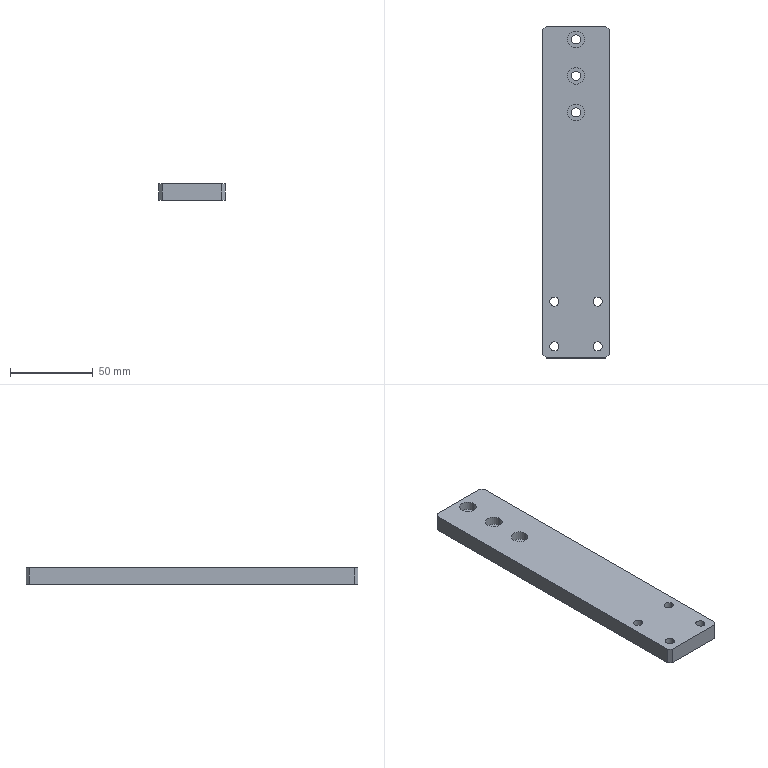Part | STEP file | 11-FG-B06111 | 1 solid | 45 faces | box 40 x 200 x 10 mm | volume 76186 mm3 | cylinder 28 | plane 17 | commonest cylinder face diameters 5.5 x14 10 x14
STEP:
#1=CARTESIAN_POINT('',(38.,7.,5.4));
#2=VERTEX_POINT('',#1);
#3=CARTESIAN_POINT('',(28.,7.,5.4));
#4=VERTEX_POINT('',#3);
#5=CARTESIAN_POINT('',(33.,7.,5.4));
#6=DIRECTION('',(0.,0.,-1.));
#7=DIRECTION('',(-1.,0.,0.));
#8=AXIS2_PLACEMENT_3D('',#5,#6,#7);
#9=CIRCLE('',#8,5.);
#10=EDGE_CURVE('',#2,#4,#9,.T.);
#11=ORIENTED_EDGE('',*,*,#10,.F.);
#12=CARTESIAN_POINT('',(38.,7.,0.));
#13=VERTEX_POINT('',#12);
#14=CARTESIAN_POINT('',(38.,7.,0.));
#15=DIRECTION('',(0.,0.,-1.));
#16=VECTOR('',#15,1000.);
#17=LINE('',#14,#16);
#18=EDGE_CURVE('',#2,#13,#17,.T.);
#19=ORIENTED_EDGE('',*,*,#18,.T.);
#20=CARTESIAN_POINT('',(28.,7.,0.));
#21=VERTEX_POINT('',#20);
#22=CARTESIAN_POINT('',(33.,7.,0.));
#23=DIRECTION('',(0.,0.,-1.));
#24=DIRECTION('',(-1.,0.,0.));
#25=AXIS2_PLACEMENT_3D('',#22,#23,#24);
#26=CIRCLE('',#25,5.);
#27=EDGE_CURVE('',#13,#21,#26,.T.);
#28=ORIENTED_EDGE('',*,*,#27,.T.);
#29=CARTESIAN_POINT('',(28.,7.,0.));
#30=DIRECTION('',(0.,0.,-1.));
#31=VECTOR('',#30,1000.);
#32=LINE('',#29,#31);
#33=EDGE_CURVE('',#4,#21,#32,.T.);
#34=ORIENTED_EDGE('',*,*,#33,.F.);
#35=EDGE_LOOP('',(#11,#19,#28,#34));
#36=FACE_OUTER_BOUND('',#35,.T.);
#37=CARTESIAN_POINT('',(33.,7.,0.));
#38=DIRECTION('',(0.,0.,-1.));
#39=DIRECTION('',(-1.,0.,0.));
#40=AXIS2_PLACEMENT_3D('',#37,#38,#39);
#41=CYLINDRICAL_SURFACE('',#40,5.);
#42=ADVANCED_FACE('',(#36),#41,.F.);
#43=CARTESIAN_POINT('',(35.75,7.,10.));
#44=VERTEX_POINT('',#43);
#45=CARTESIAN_POINT('',(30.25,7.,10.));
#46=VERTEX_POINT('',#45);
#47=CARTESIAN_POINT('',(33.,7.,10.));
#48=DIRECTION('',(0.,0.,-1.));
#49=DIRECTION('',(-1.,0.,0.));
#50=AXIS2_PLACEMENT_3D('',#47,#48,#49);
#51=CIRCLE('',#50,2.75);
#52=EDGE_CURVE('',#44,#46,#51,.T.);
#53=ORIENTED_EDGE('',*,*,#52,.F.);
#54=CARTESIAN_POINT('',(35.75,7.,5.4));
#55=VERTEX_POINT('',#54);
#56=CARTESIAN_POINT('',(35.75,7.,0.));
#57=DIRECTION('',(0.,0.,-1.));
#58=VECTOR('',#57,1000.);
#59=LINE('',#56,#58);
#60=EDGE_CURVE('',#44,#55,#59,.T.);
#61=ORIENTED_EDGE('',*,*,#60,.T.);
#62=CARTESIAN_POINT('',(30.25,7.,5.4));
#63=VERTEX_POINT('',#62);
#64=CARTESIAN_POINT('',(33.,7.,5.4));
#65=DIRECTION('',(0.,0.,-1.));
#66=DIRECTION('',(-1.,0.,0.));
#67=AXIS2_PLACEMENT_3D('',#64,#65,#66);
#68=CIRCLE('',#67,2.75);
#69=EDGE_CURVE('',#55,#63,#68,.T.);
#70=ORIENTED_EDGE('',*,*,#69,.T.);
#71=CARTESIAN_POINT('',(30.25,7.,0.));
#72=DIRECTION('',(0.,0.,-1.));
#73=VECTOR('',#72,1000.);
#74=LINE('',#71,#73);
#75=EDGE_CURVE('',#46,#63,#74,.T.);
#76=ORIENTED_EDGE('',*,*,#75,.F.);
#77=EDGE_LOOP('',(#53,#61,#70,#76));
#78=FACE_OUTER_BOUND('',#77,.T.);
#79=CARTESIAN_POINT('',(33.,7.,0.));
#80=DIRECTION('',(0.,0.,-1.));
#81=DIRECTION('',(-1.,0.,0.));
#82=AXIS2_PLACEMENT_3D('',#79,#80,#81);
#83=CYLINDRICAL_SURFACE('',#82,2.75);
#84=ADVANCED_FACE('',(#78),#83,.F.);
#85=CARTESIAN_POINT('',(12.,7.,5.4));
#86=VERTEX_POINT('',#85);
#87=CARTESIAN_POINT('',(2.,7.,5.4));
#88=VERTEX_POINT('',#87);
#89=CARTESIAN_POINT('',(7.,7.,5.4));
#90=DIRECTION('',(0.,0.,-1.));
#91=DIRECTION('',(-1.,0.,0.));
#92=AXIS2_PLACEMENT_3D('',#89,#90,#91);
#93=CIRCLE('',#92,5.);
#94=EDGE_CURVE('',#86,#88,#93,.T.);
#95=ORIENTED_EDGE('',*,*,#94,.F.);
#96=CARTESIAN_POINT('',(12.,7.,0.));
#97=VERTEX_POINT('',#96);
#98=CARTESIAN_POINT('',(12.,7.,0.));
#99=DIRECTION('',(0.,0.,-1.));
#100=VECTOR('',#99,1000.);
#101=LINE('',#98,#100);
#102=EDGE_CURVE('',#86,#97,#101,.T.);
#103=ORIENTED_EDGE('',*,*,#102,.T.);
#104=CARTESIAN_POINT('',(2.,7.,0.));
#105=VERTEX_POINT('',#104);
#106=CARTESIAN_POINT('',(7.,7.,0.));
#107=DIRECTION('',(0.,0.,-1.));
#108=DIRECTION('',(-1.,0.,0.));
#109=AXIS2_PLACEMENT_3D('',#106,#107,#108);
#110=CIRCLE('',#109,5.);
#111=EDGE_CURVE('',#97,#105,#110,.T.);
#112=ORIENTED_EDGE('',*,*,#111,.T.);
#113=CARTESIAN_POINT('',(2.,7.,0.));
#114=DIRECTION('',(0.,0.,-1.));
#115=VECTOR('',#114,1000.);
#116=LINE('',#113,#115);
#117=EDGE_CURVE('',#88,#105,#116,.T.);
#118=ORIENTED_EDGE('',*,*,#117,.F.);
#119=EDGE_LOOP('',(#95,#103,#112,#118));
#120=FACE_OUTER_BOUND('',#119,.T.);
#121=CARTESIAN_POINT('',(7.,7.,0.));
#122=DIRECTION('',(0.,0.,-1.));
#123=DIRECTION('',(-1.,0.,0.));
#124=AXIS2_PLACEMENT_3D('',#121,#122,#123);
#125=CYLINDRICAL_SURFACE('',#124,5.);
#126=ADVANCED_FACE('',(#120),#125,.F.);
#127=CARTESIAN_POINT('',(9.75,7.,10.));
#128=VERTEX_POINT('',#127);
#129=CARTESIAN_POINT('',(4.25,7.,10.));
#130=VERTEX_POINT('',#129);
#131=CARTESIAN_POINT('',(7.,7.,10.));
#132=DIRECTION('',(0.,0.,-1.));
#133=DIRECTION('',(-1.,0.,0.));
#134=AXIS2_PLACEMENT_3D('',#131,#132,#133);
#135=CIRCLE('',#134,2.75);
#136=EDGE_CURVE('',#128,#130,#135,.T.);
#137=ORIENTED_EDGE('',*,*,#136,.F.);
#138=CARTESIAN_POINT('',(9.75,7.,5.4));
#139=VERTEX_POINT('',#138);
#140=CARTESIAN_POINT('',(9.75,7.,0.));
#141=DIRECTION('',(0.,0.,-1.));
#142=VECTOR('',#141,1000.);
#143=LINE('',#140,#142);
#144=EDGE_CURVE('',#128,#139,#143,.T.);
#145=ORIENTED_EDGE('',*,*,#144,.T.);
#146=CARTESIAN_POINT('',(4.25,7.,5.4));
#147=VERTEX_POINT('',#146);
#148=CARTESIAN_POINT('',(7.,7.,5.4));
#149=DIRECTION('',(0.,0.,-1.));
#150=DIRECTION('',(-1.,0.,0.));
#151=AXIS2_PLACEMENT_3D('',#148,#149,#150);
#152=CIRCLE('',#151,2.75);
#153=EDGE_CURVE('',#139,#147,#152,.T.);
#154=ORIENTED_EDGE('',*,*,#153,.T.);
#155=CARTESIAN_POINT('',(4.25,7.,0.));
#156=DIRECTION('',(0.,0.,-1.));
#157=VECTOR('',#156,1000.);
#158=LINE('',#155,#157);
#159=EDGE_CURVE('',#130,#147,#158,.T.);
#160=ORIENTED_EDGE('',*,*,#159,.F.);
#161=EDGE_LOOP('',(#137,#145,#154,#160));
#162=FACE_OUTER_BOUND('',#161,.T.);
#163=CARTESIAN_POINT('',(7.,7.,0.));
#164=DIRECTION('',(0.,0.,-1.));
#165=DIRECTION('',(-1.,0.,0.));
#166=AXIS2_PLACEMENT_3D('',#163,#164,#165);
#167=CYLINDRICAL_SURFACE('',#166,2.75);
#168=ADVANCED_FACE('',(#162),#167,.F.);
#169=CARTESIAN_POINT('',(38.,34.,5.4));
#170=VERTEX_POINT('',#169);
#171=CARTESIAN_POINT('',(28.,34.,5.4));
#172=VERTEX_POINT('',#171);
#173=CARTESIAN_POINT('',(33.,34.,5.4));
#174=DIRECTION('',(0.,0.,-1.));
#175=DIRECTION('',(-1.,0.,0.));
#176=AXIS2_PLACEMENT_3D('',#173,#174,#175);
#177=CIRCLE('',#176,5.);
#178=EDGE_CURVE('',#170,#172,#177,.T.);
#179=ORIENTED_EDGE('',*,*,#178,.F.);
#180=CARTESIAN_POINT('',(38.,34.,0.));
#181=VERTEX_POINT('',#180);
#182=CARTESIAN_POINT('',(38.,34.,0.));
#183=DIRECTION('',(0.,0.,-1.));
#184=VECTOR('',#183,1000.);
#185=LINE('',#182,#184);
#186=EDGE_CURVE('',#170,#181,#185,.T.);
#187=ORIENTED_EDGE('',*,*,#186,.T.);
#188=CARTESIAN_POINT('',(28.,34.,0.));
#189=VERTEX_POINT('',#188);
#190=CARTESIAN_POINT('',(33.,34.,0.));
#191=DIRECTION('',(0.,0.,-1.));
#192=DIRECTION('',(-1.,0.,0.));
#193=AXIS2_PLACEMENT_3D('',#190,#191,#192);
#194=CIRCLE('',#193,5.);
#195=EDGE_CURVE('',#181,#189,#194,.T.);
#196=ORIENTED_EDGE('',*,*,#195,.T.);
#197=CARTESIAN_POINT('',(28.,34.,0.));
#198=DIRECTION('',(0.,0.,-1.));
#199=VECTOR('',#198,1000.);
#200=LINE('',#197,#199);
#201=EDGE_CURVE('',#172,#189,#200,.T.);
#202=ORIENTED_EDGE('',*,*,#201,.F.);
#203=EDGE_LOOP('',(#179,#187,#196,#202));
#204=FACE_OUTER_BOUND('',#203,.T.);
#205=CARTESIAN_POINT('',(33.,34.,0.));
#206=DIRECTION('',(0.,0.,-1.));
#207=DIRECTION('',(-1.,0.,0.));
#208=AXIS2_PLACEMENT_3D('',#205,#206,#207);
#209=CYLINDRICAL_SURFACE('',#208,5.);
#210=ADVANCED_FACE('',(#204),#209,.F.);
#211=CARTESIAN_POINT('',(35.75,34.,10.));
#212=VERTEX_POINT('',#211);
#213=CARTESIAN_POINT('',(30.25,34.,10.));
#214=VERTEX_POINT('',#213);
#215=CARTESIAN_POINT('',(33.,34.,10.));
#216=DIRECTION('',(0.,0.,-1.));
#217=DIRECTION('',(-1.,0.,0.));
#218=AXIS2_PLACEMENT_3D('',#215,#216,#217);
#219=CIRCLE('',#218,2.75);
#220=EDGE_CURVE('',#212,#214,#219,.T.);
#221=ORIENTED_EDGE('',*,*,#220,.F.);
#222=CARTESIAN_POINT('',(35.75,34.,5.4));
#223=VERTEX_POINT('',#222);
#224=CARTESIAN_POINT('',(35.75,34.,0.));
#225=DIRECTION('',(0.,0.,-1.));
#226=VECTOR('',#225,1000.);
#227=LINE('',#224,#226);
#228=EDGE_CURVE('',#212,#223,#227,.T.);
#229=ORIENTED_EDGE('',*,*,#228,.T.);
#230=CARTESIAN_POINT('',(30.25,34.,5.4));
#231=VERTEX_POINT('',#230);
#232=CARTESIAN_POINT('',(33.,34.,5.4));
#233=DIRECTION('',(0.,0.,-1.));
#234=DIRECTION('',(-1.,0.,0.));
#235=AXIS2_PLACEMENT_3D('',#232,#233,#234);
#236=CIRCLE('',#235,2.75);
#237=EDGE_CURVE('',#223,#231,#236,.T.);
#238=ORIENTED_EDGE('',*,*,#237,.T.);
#239=CARTESIAN_POINT('',(30.25,34.,0.));
#240=DIRECTION('',(0.,0.,-1.));
#241=VECTOR('',#240,1000.);
#242=LINE('',#239,#241);
#243=EDGE_CURVE('',#214,#231,#242,.T.);
#244=ORIENTED_EDGE('',*,*,#243,.F.);
#245=EDGE_LOOP('',(#221,#229,#238,#244));
#246=FACE_OUTER_BOUND('',#245,.T.);
#247=CARTESIAN_POINT('',(33.,34.,0.));
#248=DIRECTION('',(0.,0.,-1.));
#249=DIRECTION('',(-1.,0.,0.));
#250=AXIS2_PLACEMENT_3D('',#247,#248,#249);
#251=CYLINDRICAL_SURFACE('',#250,2.75);
#252=ADVANCED_FACE('',(#246),#251,.F.);
#253=CARTESIAN_POINT('',(12.,34.,5.4));
#254=VERTEX_POINT('',#253);
#255=CARTESIAN_POINT('',(2.,34.,5.4));
#256=VERTEX_POINT('',#255);
#257=CARTESIAN_POINT('',(7.,34.,5.4));
#258=DIRECTION('',(0.,0.,-1.));
#259=DIRECTION('',(-1.,0.,0.));
#260=AXIS2_PLACEMENT_3D('',#257,#258,#259);
#261=CIRCLE('',#260,5.);
#262=EDGE_CURVE('',#254,#256,#261,.T.);
#263=ORIENTED_EDGE('',*,*,#262,.F.);
#264=CARTESIAN_POINT('',(12.,34.,0.));
#265=VERTEX_POINT('',#264);
#266=CARTESIAN_POINT('',(12.,34.,0.));
#267=DIRECTION('',(0.,0.,-1.));
#268=VECTOR('',#267,1000.);
#269=LINE('',#266,#268);
#270=EDGE_CURVE('',#254,#265,#269,.T.);
#271=ORIENTED_EDGE('',*,*,#270,.T.);
#272=CARTESIAN_POINT('',(2.,34.,0.));
#273=VERTEX_POINT('',#272);
#274=CARTESIAN_POINT('',(7.,34.,0.));
#275=DIRECTION('',(0.,0.,-1.));
#276=DIRECTION('',(-1.,0.,0.));
#277=AXIS2_PLACEMENT_3D('',#274,#275,#276);
#278=CIRCLE('',#277,5.);
#279=EDGE_CURVE('',#265,#273,#278,.T.);
#280=ORIENTED_EDGE('',*,*,#279,.T.);
#281=CARTESIAN_POINT('',(2.,34.,0.));
#282=DIRECTION('',(0.,0.,-1.));
#283=VECTOR('',#282,1000.);
#284=LINE('',#281,#283);
#285=EDGE_CURVE('',#256,#273,#284,.T.);
#286=ORIENTED_EDGE('',*,*,#285,.F.);
#287=EDGE_LOOP('',(#263,#271,#280,#286));
#288=FACE_OUTER_BOUND('',#287,.T.);
#289=CARTESIAN_POINT('',(7.,34.,0.));
#290=DIRECTION('',(0.,0.,-1.));
#291=DIRECTION('',(-1.,0.,0.));
#292=AXIS2_PLACEMENT_3D('',#289,#290,#291);
#293=CYLINDRICAL_SURFACE('',#292,5.);
#294=ADVANCED_FACE('',(#288),#293,.F.);
#295=CARTESIAN_POINT('',(9.75,34.,10.));
#296=VERTEX_POINT('',#295);
#297=CARTESIAN_POINT('',(4.25,34.,10.));
#298=VERTEX_POINT('',#297);
#299=CARTESIAN_POINT('',(7.,34.,10.));
#300=DIRECTION('',(0.,0.,-1.));
#301=DIRECTION('',(-1.,0.,0.));
#302=AXIS2_PLACEMENT_3D('',#299,#300,#301);
#303=CIRCLE('',#302,2.75);
#304=EDGE_CURVE('',#296,#298,#303,.T.);
#305=ORIENTED_EDGE('',*,*,#304,.F.);
#306=CARTESIAN_POINT('',(9.75,34.,5.4));
#307=VERTEX_POINT('',#306);
#308=CARTESIAN_POINT('',(9.75,34.,0.));
#309=DIRECTION('',(0.,0.,-1.));
#310=VECTOR('',#309,1000.);
#311=LINE('',#308,#310);
#312=EDGE_CURVE('',#296,#307,#311,.T.);
#313=ORIENTED_EDGE('',*,*,#312,.T.);
#314=CARTESIAN_POINT('',(4.25,34.,5.4));
#315=VERTEX_POINT('',#314);
#316=CARTESIAN_POINT('',(7.,34.,5.4));
#317=DIRECTION('',(0.,0.,-1.));
#318=DIRECTION('',(-1.,0.,0.));
#319=AXIS2_PLACEMENT_3D('',#316,#317,#318);
#320=CIRCLE('',#319,2.75);
#321=EDGE_CURVE('',#307,#315,#320,.T.);
#322=ORIENTED_EDGE('',*,*,#321,.T.);
#323=CARTESIAN_POINT('',(4.25,34.,0.));
#324=DIRECTION('',(0.,0.,-1.));
#325=VECTOR('',#324,1000.);
#326=LINE('',#323,#325);
#327=EDGE_CURVE('',#298,#315,#326,.T.);
#328=ORIENTED_EDGE('',*,*,#327,.F.);
#329=EDGE_LOOP('',(#305,#313,#322,#328));
#330=FACE_OUTER_BOUND('',#329,.T.);
#331=CARTESIAN_POINT('',(7.,34.,0.));
#332=DIRECTION('',(0.,0.,-1.));
#333=DIRECTION('',(-1.,0.,0.));
#334=AXIS2_PLACEMENT_3D('',#331,#332,#333);
#335=CYLINDRICAL_SURFACE('',#334,2.75);
#336=ADVANCED_FACE('',(#330),#335,.F.);
#337=CARTESIAN_POINT('',(15.,148.,4.6));
#338=VERTEX_POINT('',#337);
#339=CARTESIAN_POINT('',(25.,148.,4.6));
#340=VERTEX_POINT('',#339);
#341=CARTESIAN_POINT('',(20.,148.,4.6));
#342=DIRECTION('',(0.,0.,1.));
#343=DIRECTION('',(1.,0.,0.));
#344=AXIS2_PLACEMENT_3D('',#341,#342,#343);
#345=CIRCLE('',#344,5.);
#346=EDGE_CURVE('',#338,#340,#345,.T.);
#347=ORIENTED_EDGE('',*,*,#346,.F.);
#348=CARTESIAN_POINT('',(15.,148.,10.));
#349=VERTEX_POINT('',#348);
#350=CARTESIAN_POINT('',(15.,148.,10.));
#351=DIRECTION('',(0.,0.,1.));
#352=VECTOR('',#351,1000.);
#353=LINE('',#350,#352);
#354=EDGE_CURVE('',#338,#349,#353,.T.);
#355=ORIENTED_EDGE('',*,*,#354,.T.);
#356=CARTESIAN_POINT('',(25.,148.,10.));
#357=VERTEX_POINT('',#356);
#358=CARTESIAN_POINT('',(20.,148.,10.));
#359=DIRECTION('',(0.,0.,1.));
#360=DIRECTION('',(1.,0.,0.));
#361=AXIS2_PLACEMENT_3D('',#358,#359,#360);
#362=CIRCLE('',#361,5.);
#363=EDGE_CURVE('',#349,#357,#362,.T.);
#364=ORIENTED_EDGE('',*,*,#363,.T.);
#365=CARTESIAN_POINT('',(25.,148.,10.));
#366=DIRECTION('',(0.,0.,1.));
#367=VECTOR('',#366,1000.);
#368=LINE('',#365,#367);
#369=EDGE_CURVE('',#340,#357,#368,.T.);
#370=ORIENTED_EDGE('',*,*,#369,.F.);
#371=EDGE_LOOP('',(#347,#355,#364,#370));
#372=FACE_OUTER_BOUND('',#371,.T.);
#373=CARTESIAN_POINT('',(20.,148.,10.));
#374=DIRECTION('',(0.,0.,1.));
#375=DIRECTION('',(1.,0.,0.));
#376=AXIS2_PLACEMENT_3D('',#373,#374,#375);
#377=CYLINDRICAL_SURFACE('',#376,5.);
#378=ADVANCED_FACE('',(#372),#377,.F.);
#379=CARTESIAN_POINT('',(22.75,148.,0.));
#380=VERTEX_POINT('',#379);
#381=CARTESIAN_POINT('',(17.25,148.,0.));
#382=VERTEX_POINT('',#381);
#383=CARTESIAN_POINT('',(20.,148.,0.));
#384=DIRECTION('',(0.,0.,-1.));
#385=DIRECTION('',(-1.,0.,0.));
#386=AXIS2_PLACEMENT_3D('',#383,#384,#385);
#387=CIRCLE('',#386,2.75);
#388=EDGE_CURVE('',#380,#382,#387,.T.);
#389=ORIENTED_EDGE('',*,*,#388,.T.);
#390=CARTESIAN_POINT('',(17.25,148.,4.6));
#391=VERTEX_POINT('',#390);
#392=CARTESIAN_POINT('',(17.25,148.,10.));
#393=DIRECTION('',(0.,0.,1.));
#394=VECTOR('',#393,1000.);
#395=LINE('',#392,#394);
#396=EDGE_CURVE('',#382,#391,#395,.T.);
#397=ORIENTED_EDGE('',*,*,#396,.T.);
#398=CARTESIAN_POINT('',(22.75,148.,4.6));
#399=VERTEX_POINT('',#398);
#400=CARTESIAN_POINT('',(20.,148.,4.6));
#401=DIRECTION('',(0.,0.,1.));
#402=DIRECTION('',(1.,0.,0.));
#403=AXIS2_PLACEMENT_3D('',#400,#401,#402);
#404=CIRCLE('',#403,2.75);
#405=EDGE_CURVE('',#391,#399,#404,.T.);
#406=ORIENTED_EDGE('',*,*,#405,.T.);
#407=CARTESIAN_POINT('',(22.75,148.,10.));
#408=DIRECTION('',(0.,0.,1.));
#409=VECTOR('',#408,1000.);
#410=LINE('',#407,#409);
#411=EDGE_CURVE('',#380,#399,#410,.T.);
#412=ORIENTED_EDGE('',*,*,#411,.F.);
#413=EDGE_LOOP('',(#389,#397,#406,#412));
#414=FACE_OUTER_BOUND('',#413,.T.);
#415=CARTESIAN_POINT('',(20.,148.,10.));
#416=DIRECTION('',(0.,0.,1.));
#417=DIRECTION('',(1.,0.,0.));
#418=AXIS2_PLACEMENT_3D('',#415,#416,#417);
#419=CYLINDRICAL_SURFACE('',#418,2.75);
#420=ADVANCED_FACE('',(#414),#419,.F.);
#421=CARTESIAN_POINT('',(15.,170.,4.6));
#422=VERTEX_POINT('',#421);
#423=CARTESIAN_POINT('',(25.,170.,4.6));
#424=VERTEX_POINT('',#423);
#425=CARTESIAN_POINT('',(20.,170.,4.6));
#426=DIRECTION('',(0.,0.,1.));
#427=DIRECTION('',(1.,0.,0.));
#428=AXIS2_PLACEMENT_3D('',#425,#426,#427);
#429=CIRCLE('',#428,5.);
#430=EDGE_CURVE('',#422,#424,#429,.T.);
#431=ORIENTED_EDGE('',*,*,#430,.F.);
#432=CARTESIAN_POINT('',(15.,170.,10.));
#433=VERTEX_POINT('',#432);
#434=CARTESIAN_POINT('',(15.,170.,10.));
#435=DIRECTION('',(0.,0.,1.));
#436=VECTOR('',#435,1000.);
#437=LINE('',#434,#436);
#438=EDGE_CURVE('',#422,#433,#437,.T.);
#439=ORIENTED_EDGE('',*,*,#438,.T.);
#440=CARTESIAN_POINT('',(25.,170.,10.));
#441=VERTEX_POINT('',#440);
#442=CARTESIAN_POINT('',(20.,170.,10.));
#443=DIRECTION('',(0.,0.,1.));
#444=DIRECTION('',(1.,0.,0.));
#445=AXIS2_PLACEMENT_3D('',#442,#443,#444);
#446=CIRCLE('',#445,5.);
#447=EDGE_CURVE('',#433,#441,#446,.T.);
#448=ORIENTED_EDGE('',*,*,#447,.T.);
#449=CARTESIAN_POINT('',(25.,170.,10.));
#450=DIRECTION('',(0.,0.,1.));
#451=VECTOR('',#450,1000.);
#452=LINE('',#449,#451);
#453=EDGE_CURVE('',#424,#441,#452,.T.);
#454=ORIENTED_EDGE('',*,*,#453,.F.);
#455=EDGE_LOOP('',(#431,#439,#448,#454));
#456=FACE_OUTER_BOUND('',#455,.T.);
#457=CARTESIAN_POINT('',(20.,170.,10.));
#458=DIRECTION('',(0.,0.,1.));
#459=DIRECTION('',(1.,0.,0.));
#460=AXIS2_PLACEMENT_3D('',#457,#458,#459);
#461=CYLINDRICAL_SURFACE('',#460,5.);
#462=ADVANCED_FACE('',(#456),#461,.F.);
#463=CARTESIAN_POINT('',(22.75,170.,0.));
#464=VERTEX_POINT('',#463);
#465=CARTESIAN_POINT('',(17.25,170.,0.));
#466=VERTEX_POINT('',#465);
#467=CARTESIAN_POINT('',(20.,170.,0.));
#468=DIRECTION('',(0.,0.,-1.));
#469=DIRECTION('',(-1.,0.,0.));
#470=AXIS2_PLACEMENT_3D('',#467,#468,#469);
#471=CIRCLE('',#470,2.75);
#472=EDGE_CURVE('',#464,#466,#471,.T.);
#473=ORIENTED_EDGE('',*,*,#472,.T.);
#474=CARTESIAN_POINT('',(17.25,170.,4.6));
#475=VERTEX_POINT('',#474);
#476=CARTESIAN_POINT('',(17.25,170.,10.));
#477=DIRECTION('',(0.,0.,1.));
#478=VECTOR('',#477,1000.);
#479=LINE('',#476,#478);
#480=EDGE_CURVE('',#466,#475,#479,.T.);
#481=ORIENTED_EDGE('',*,*,#480,.T.);
#482=CARTESIAN_POINT('',(22.75,170.,4.6));
#483=VERTEX_POINT('',#482);
#484=CARTESIAN_POINT('',(20.,170.,4.6));
#485=DIRECTION('',(0.,0.,1.));
#486=DIRECTION('',(1.,0.,0.));
#487=AXIS2_PLACEMENT_3D('',#484,#485,#486);
#488=CIRCLE('',#487,2.75);
#489=EDGE_CURVE('',#475,#483,#488,.T.);
#490=ORIENTED_EDGE('',*,*,#489,.T.);
#491=CARTESIAN_POINT('',(22.75,170.,10.));
#492=DIRECTION('',(0.,0.,1.));
#493=VECTOR('',#492,1000.);
#494=LINE('',#491,#493);
#495=EDGE_CURVE('',#464,#483,#494,.T.);
#496=ORIENTED_EDGE('',*,*,#495,.F.);
#497=EDGE_LOOP('',(#473,#481,#490,#496));
#498=FACE_OUTER_BOUND('',#497,.T.);
#499=CARTESIAN_POINT('',(20.,170.,10.));
#500=DIRECTION('',(0.,0.,1.));
#501=DIRECTION('',(1.,0.,0.));
#502=AXIS2_PLACEMENT_3D('',#499,#500,#501);
#503=CYLINDRICAL_SURFACE('',#502,2.75);
#504=ADVANCED_FACE('',(#498),#503,.F.);
#505=CARTESIAN_POINT('',(15.,192.,4.6));
#506=VERTEX_POINT('',#505);
#507=CARTESIAN_POINT('',(25.,192.,4.6));
#508=VERTEX_POINT('',#507);
#509=CARTESIAN_POINT('',(20.,192.,4.6));
#510=DIRECTION('',(0.,0.,1.));
#511=DIRECTION('',(1.,0.,0.));
#512=AXIS2_PLACEMENT_3D('',#509,#510,#511);
#513=CIRCLE('',#512,5.);
#514=EDGE_CURVE('',#506,#508,#513,.T.);
#515=ORIENTED_EDGE('',*,*,#514,.F.);
#516=CARTESIAN_POINT('',(15.,192.,10.));
#517=VERTEX_POINT('',#516);
#518=CARTESIAN_POINT('',(15.,192.,10.));
#519=DIRECTION('',(0.,0.,1.));
#520=VECTOR('',#519,1000.);
#521=LINE('',#518,#520);
#522=EDGE_CURVE('',#506,#517,#521,.T.);
#523=ORIENTED_EDGE('',*,*,#522,.T.);
#524=CARTESIAN_POINT('',(25.,192.,10.));
#525=VERTEX_POINT('',#524);
#526=CARTESIAN_POINT('',(20.,192.,10.));
#527=DIRECTION('',(0.,0.,1.));
#528=DIRECTION('',(1.,0.,0.));
#529=AXIS2_PLACEMENT_3D('',#526,#527,#528);
#530=CIRCLE('',#529,5.);
#531=EDGE_CURVE('',#517,#525,#530,.T.);
#532=ORIENTED_EDGE('',*,*,#531,.T.);
#533=CARTESIAN_POINT('',(25.,192.,10.));
#534=DIRECTION('',(0.,0.,1.));
#535=VECTOR('',#534,1000.);
#536=LINE('',#533,#535);
#537=EDGE_CURVE('',#508,#525,#536,.T.);
#538=ORIENTED_EDGE('',*,*,#537,.F.);
#539=EDGE_LOOP('',(#515,#523,#532,#538));
#540=FACE_OUTER_BOUND('',#539,.T.);
#541=CARTESIAN_POINT('',(20.,192.,10.));
#542=DIRECTION('',(0.,0.,1.));
#543=DIRECTION('',(1.,0.,0.));
#544=AXIS2_PLACEMENT_3D('',#541,#542,#543);
#545=CYLINDRICAL_SURFACE('',#544,5.);
#546=ADVANCED_FACE('',(#540),#545,.F.);
#547=CARTESIAN_POINT('',(22.75,192.,0.));
#548=VERTEX_POINT('',#547);
#549=CARTESIAN_POINT('',(17.25,192.,0.));
#550=VERTEX_POINT('',#549);
#551=CARTESIAN_POINT('',(20.,192.,0.));
#552=DIRECTION('',(0.,0.,-1.));
#553=DIRECTION('',(-1.,0.,0.));
#554=AXIS2_PLACEMENT_3D('',#551,#552,#553);
#555=CIRCLE('',#554,2.75);
#556=EDGE_CURVE('',#548,#550,#555,.T.);
#557=ORIENTED_EDGE('',*,*,#556,.T.);
#558=CARTESIAN_POINT('',(17.25,192.,4.6));
#559=VERTEX_POINT('',#558);
#560=CARTESIAN_POINT('',(17.25,192.,10.));
#561=DIRECTION('',(0.,0.,1.));
#562=VECTOR('',#561,1000.);
#563=LINE('',#560,#562);
#564=EDGE_CURVE('',#550,#559,#563,.T.);
#565=ORIENTED_EDGE('',*,*,#564,.T.);
#566=CARTESIAN_POINT('',(22.75,192.,4.6));
#567=VERTEX_POINT('',#566);
#568=CARTESIAN_POINT('',(20.,192.,4.6));
#569=DIRECTION('',(0.,0.,1.));
#570=DIRECTION('',(1.,0.,0.));
#571=AXIS2_PLACEMENT_3D('',#568,#569,#570);
#572=CIRCLE('',#571,2.75);
#573=EDGE_CURVE('',#559,#567,#572,.T.);
#574=ORIENTED_EDGE('',*,*,#573,.T.);
#575=CARTESIAN_POINT('',(22.75,192.,10.));
#576=DIRECTION('',(0.,0.,1.));
#577=VECTOR('',#576,1000.);
#578=LINE('',#575,#577);
#579=EDGE_CURVE('',#548,#567,#578,.T.);
#580=ORIENTED_EDGE('',*,*,#579,.F.);
#581=EDGE_LOOP('',(#557,#565,#574,#580));
#582=FACE_OUTER_BOUND('',#581,.T.);
#583=CARTESIAN_POINT('',(20.,192.,10.));
#584=DIRECTION('',(0.,0.,1.));
#585=DIRECTION('',(1.,0.,0.));
#586=AXIS2_PLACEMENT_3D('',#583,#584,#585);
#587=CYLINDRICAL_SURFACE('',#586,2.75);
#588=ADVANCED_FACE('',(#582),#587,.F.);
#589=CARTESIAN_POINT('',(0.,198.,0.));
#590=VERTEX_POINT('',#589);
#591=CARTESIAN_POINT('',(0.,2.,0.));
#592=VERTEX_POINT('',#591);
#593=CARTESIAN_POINT('',(0.,0.,0.));
#594=DIRECTION('',(0.,-1.,0.));
#595=VECTOR('',#594,1000.);
#596=LINE('',#593,#595);
#597=EDGE_CURVE('',#590,#592,#596,.T.);
#598=ORIENTED_EDGE('',*,*,#597,.T.);
#599=CARTESIAN_POINT('',(0.,2.,10.));
#600=VERTEX_POINT('',#599);
#601=CARTESIAN_POINT('',(0.,2.,10.));
#602=DIRECTION('',(0.,0.,1.));
#603=VECTOR('',#602,1000.);
#604=LINE('',#601,#603);
#605=EDGE_CURVE('',#592,#600,#604,.T.);
#606=ORIENTED_EDGE('',*,*,#605,.T.);
#607=CARTESIAN_POINT('',(0.,198.,10.));
#608=VERTEX_POINT('',#607);
#609=CARTESIAN_POINT('',(0.,0.,10.));
#610=DIRECTION('',(0.,-1.,0.));
#611=VECTOR('',#610,1000.);
#612=LINE('',#609,#611);
#613=EDGE_CURVE('',#608,#600,#612,.T.);
#614=ORIENTED_EDGE('',*,*,#613,.F.);
#615=CARTESIAN_POINT('',(0.,198.,10.));
#616=DIRECTION('',(0.,0.,-1.));
#617=VECTOR('',#616,1000.);
#618=LINE('',#615,#617);
#619=EDGE_CURVE('',#608,#590,#618,.T.);
#620=ORIENTED_EDGE('',*,*,#619,.T.);
#621=EDGE_LOOP('',(#598,#606,#614,#620));
#622=FACE_OUTER_BOUND('',#621,.T.);
#623=CARTESIAN_POINT('',(0.,0.,10.));
#624=DIRECTION('',(1.,0.,0.));
#625=DIRECTION('',(0.,1.,0.));
#626=AXIS2_PLACEMENT_3D('',#623,#624,#625);
#627=PLANE('',#626);
#628=ADVANCED_FACE('',(#622),#627,.F.);
#629=CARTESIAN_POINT('',(2.,0.,10.));
#630=VERTEX_POINT('',#629);
#631=CARTESIAN_POINT('',(38.,0.,10.));
#632=VERTEX_POINT('',#631);
#633=CARTESIAN_POINT('',(0.,0.,10.));
#634=DIRECTION('',(1.,0.,0.));
#635=VECTOR('',#634,1000.);
#636=LINE('',#633,#635);
#637=EDGE_CURVE('',#630,#632,#636,.T.);
#638=ORIENTED_EDGE('',*,*,#637,.F.);
#639=CARTESIAN_POINT('',(2.,0.,0.));
#640=VERTEX_POINT('',#639);
#641=CARTESIAN_POINT('',(2.,0.,10.));
#642=DIRECTION('',(0.,0.,-1.));
#643=VECTOR('',#642,1000.);
#644=LINE('',#641,#643);
#645=EDGE_CURVE('',#630,#640,#644,.T.);
#646=ORIENTED_EDGE('',*,*,#645,.T.);
#647=CARTESIAN_POINT('',(38.,0.,0.));
#648=VERTEX_POINT('',#647);
#649=CARTESIAN_POINT('',(0.,0.,0.));
#650=DIRECTION('',(1.,0.,0.));
#651=VECTOR('',#650,1000.);
#652=LINE('',#649,#651);
#653=EDGE_CURVE('',#640,#648,#652,.T.);
#654=ORIENTED_EDGE('',*,*,#653,.T.);
#655=CARTESIAN_POINT('',(38.,0.,10.));
#656=DIRECTION('',(0.,0.,1.));
#657=VECTOR('',#656,1000.);
#658=LINE('',#655,#657);
#659=EDGE_CURVE('',#648,#632,#658,.T.);
#660=ORIENTED_EDGE('',*,*,#659,.T.);
#661=EDGE_LOOP('',(#638,#646,#654,#660));
#662=FACE_OUTER_BOUND('',#661,.T.);
#663=CARTESIAN_POINT('',(0.,0.,10.));
#664=DIRECTION('',(0.,1.,0.));
#665=DIRECTION('',(0.,0.,1.));
#666=AXIS2_PLACEMENT_3D('',#663,#664,#665);
#667=PLANE('',#666);
#668=ADVANCED_FACE('',(#662),#667,.F.);
#669=CARTESIAN_POINT('',(40.,2.,10.));
#670=VERTEX_POINT('',#669);
#671=CARTESIAN_POINT('',(40.,198.,10.));
#672=VERTEX_POINT('',#671);
#673=CARTESIAN_POINT('',(40.,200.,10.));
#674=DIRECTION('',(0.,1.,0.));
#675=VECTOR('',#674,1000.);
#676=LINE('',#673,#675);
#677=EDGE_CURVE('',#670,#672,#676,.T.);
#678=ORIENTED_EDGE('',*,*,#677,.F.);
#679=CARTESIAN_POINT('',(40.,2.,0.));
#680=VERTEX_POINT('',#679);
#681=CARTESIAN_POINT('',(40.,2.,10.));
#682=DIRECTION('',(0.,0.,-1.));
#683=VECTOR('',#682,1000.);
#684=LINE('',#681,#683);
#685=EDGE_CURVE('',#670,#680,#684,.T.);
#686=ORIENTED_EDGE('',*,*,#685,.T.);
#687=CARTESIAN_POINT('',(40.,198.,0.));
#688=VERTEX_POINT('',#687);
#689=CARTESIAN_POINT('',(40.,200.,0.));
#690=DIRECTION('',(0.,1.,0.));
#691=VECTOR('',#690,1000.);
#692=LINE('',#689,#691);
#693=EDGE_CURVE('',#680,#688,#692,.T.);
#694=ORIENTED_EDGE('',*,*,#693,.T.);
#695=CARTESIAN_POINT('',(40.,198.,10.));
#696=DIRECTION('',(0.,0.,1.));
#697=VECTOR('',#696,1000.);
#698=LINE('',#695,#697);
#699=EDGE_CURVE('',#688,#672,#698,.T.);
#700=ORIENTED_EDGE('',*,*,#699,.T.);
#701=EDGE_LOOP('',(#678,#686,#694,#700));
#702=FACE_OUTER_BOUND('',#701,.T.);
#703=CARTESIAN_POINT('',(40.,200.,10.));
#704=DIRECTION('',(-1.,0.,0.));
#705=DIRECTION('',(0.,-1.,0.));
#706=AXIS2_PLACEMENT_3D('',#703,#704,#705);
#707=PLANE('',#706);
#708=ADVANCED_FACE('',(#702),#707,.F.);
#709=CARTESIAN_POINT('',(38.,200.,10.));
#710=VERTEX_POINT('',#709);
#711=CARTESIAN_POINT('',(2.,200.,10.));
#712=VERTEX_POINT('',#711);
#713=CARTESIAN_POINT('',(0.,200.,10.));
#714=DIRECTION('',(-1.,0.,0.));
#715=VECTOR('',#714,1000.);
#716=LINE('',#713,#715);
#717=EDGE_CURVE('',#710,#712,#716,.T.);
#718=ORIENTED_EDGE('',*,*,#717,.F.);
#719=CARTESIAN_POINT('',(38.,200.,0.));
#720=VERTEX_POINT('',#719);
#721=CARTESIAN_POINT('',(38.,200.,10.));
#722=DIRECTION('',(0.,0.,-1.));
#723=VECTOR('',#722,1000.);
#724=LINE('',#721,#723);
#725=EDGE_CURVE('',#710,#720,#724,.T.);
#726=ORIENTED_EDGE('',*,*,#725,.T.);
#727=CARTESIAN_POINT('',(2.,200.,0.));
#728=VERTEX_POINT('',#727);
#729=CARTESIAN_POINT('',(0.,200.,0.));
#730=DIRECTION('',(-1.,0.,0.));
#731=VECTOR('',#730,1000.);
#732=LINE('',#729,#731);
#733=EDGE_CURVE('',#720,#728,#732,.T.);
#734=ORIENTED_EDGE('',*,*,#733,.T.);
#735=CARTESIAN_POINT('',(2.,200.,10.));
#736=DIRECTION('',(0.,0.,1.));
#737=VECTOR('',#736,1000.);
#738=LINE('',#735,#737);
#739=EDGE_CURVE('',#728,#712,#738,.T.);
#740=ORIENTED_EDGE('',*,*,#739,.T.);
#741=EDGE_LOOP('',(#718,#726,#734,#740));
#742=FACE_OUTER_BOUND('',#741,.T.);
#743=CARTESIAN_POINT('',(0.,200.,10.));
#744=DIRECTION('',(0.,-1.,0.));
#745=DIRECTION('',(0.,0.,-1.));
#746=AXIS2_PLACEMENT_3D('',#743,#744,#745);
#747=PLANE('',#746);
#748=ADVANCED_FACE('',(#742),#747,.F.);
#749=CARTESIAN_POINT('',(33.,7.,10.));
#750=DIRECTION('',(0.,0.,-1.));
#751=DIRECTION('',(-1.,0.,0.));
#752=AXIS2_PLACEMENT_3D('',#749,#750,#751);
#753=CIRCLE('',#752,2.75);
#754=EDGE_CURVE('',#46,#44,#753,.T.);
#755=ORIENTED_EDGE('',*,*,#754,.T.);
#756=ORIENTED_EDGE('',*,*,#52,.T.);
#757=EDGE_LOOP('',(#755,#756));
#758=FACE_BOUND('',#757,.T.);
#759=CARTESIAN_POINT('',(7.,7.,10.));
#760=DIRECTION('',(0.,0.,-1.));
#761=DIRECTION('',(-1.,0.,0.));
#762=AXIS2_PLACEMENT_3D('',#759,#760,#761);
#763=CIRCLE('',#762,2.75);
#764=EDGE_CURVE('',#130,#128,#763,.T.);
#765=ORIENTED_EDGE('',*,*,#764,.T.);
#766=ORIENTED_EDGE('',*,*,#136,.T.);
#767=EDGE_LOOP('',(#765,#766));
#768=FACE_BOUND('',#767,.T.);
#769=CARTESIAN_POINT('',(33.,34.,10.));
#770=DIRECTION('',(0.,0.,-1.));
#771=DIRECTION('',(-1.,0.,0.));
#772=AXIS2_PLACEMENT_3D('',#769,#770,#771);
#773=CIRCLE('',#772,2.75);
#774=EDGE_CURVE('',#214,#212,#773,.T.);
#775=ORIENTED_EDGE('',*,*,#774,.T.);
#776=ORIENTED_EDGE('',*,*,#220,.T.);
#777=EDGE_LOOP('',(#775,#776));
#778=FACE_BOUND('',#777,.T.);
#779=CARTESIAN_POINT('',(7.,34.,10.));
#780=DIRECTION('',(0.,0.,-1.));
#781=DIRECTION('',(-1.,0.,0.));
#782=AXIS2_PLACEMENT_3D('',#779,#780,#781);
#783=CIRCLE('',#782,2.75);
#784=EDGE_CURVE('',#298,#296,#783,.T.);
#785=ORIENTED_EDGE('',*,*,#784,.T.);
#786=ORIENTED_EDGE('',*,*,#304,.T.);
#787=EDGE_LOOP('',(#785,#786));
#788=FACE_BOUND('',#787,.T.);
#789=CARTESIAN_POINT('',(20.,148.,10.));
#790=DIRECTION('',(0.,0.,1.));
#791=DIRECTION('',(1.,0.,0.));
#792=AXIS2_PLACEMENT_3D('',#789,#790,#791);
#793=CIRCLE('',#792,5.);
#794=EDGE_CURVE('',#357,#349,#793,.T.);
#795=ORIENTED_EDGE('',*,*,#794,.F.);
#796=ORIENTED_EDGE('',*,*,#363,.F.);
#797=EDGE_LOOP('',(#795,#796));
#798=FACE_BOUND('',#797,.T.);
#799=CARTESIAN_POINT('',(20.,170.,10.));
#800=DIRECTION('',(0.,0.,1.));
#801=DIRECTION('',(1.,0.,0.));
#802=AXIS2_PLACEMENT_3D('',#799,#800,#801);
#803=CIRCLE('',#802,5.);
#804=EDGE_CURVE('',#441,#433,#803,.T.);
#805=ORIENTED_EDGE('',*,*,#804,.F.);
#806=ORIENTED_EDGE('',*,*,#447,.F.);
#807=EDGE_LOOP('',(#805,#806));
#808=FACE_BOUND('',#807,.T.);
#809=CARTESIAN_POINT('',(20.,192.,10.));
#810=DIRECTION('',(0.,0.,1.));
#811=DIRECTION('',(1.,0.,0.));
#812=AXIS2_PLACEMENT_3D('',#809,#810,#811);
#813=CIRCLE('',#812,5.);
#814=EDGE_CURVE('',#525,#517,#813,.T.);
#815=ORIENTED_EDGE('',*,*,#814,.F.);
#816=ORIENTED_EDGE('',*,*,#531,.F.);
#817=EDGE_LOOP('',(#815,#816));
#818=FACE_BOUND('',#817,.T.);
#819=ORIENTED_EDGE('',*,*,#613,.T.);
#820=CARTESIAN_POINT('',(2.,0.,10.));
#821=DIRECTION('',(0.7071,-0.7071,0.));
#822=VECTOR('',#821,1000.);
#823=LINE('',#820,#822);
#824=EDGE_CURVE('',#600,#630,#823,.T.);
#825=ORIENTED_EDGE('',*,*,#824,.T.);
#826=ORIENTED_EDGE('',*,*,#637,.T.);
#827=CARTESIAN_POINT('',(40.,2.,10.));
#828=DIRECTION('',(0.7071,0.7071,0.));
#829=VECTOR('',#828,1000.);
#830=LINE('',#827,#829);
#831=EDGE_CURVE('',#632,#670,#830,.T.);
#832=ORIENTED_EDGE('',*,*,#831,.T.);
#833=ORIENTED_EDGE('',*,*,#677,.T.);
#834=CARTESIAN_POINT('',(38.,200.,10.));
#835=DIRECTION('',(-0.7071,0.7071,0.));
#836=VECTOR('',#835,1000.);
#837=LINE('',#834,#836);
#838=EDGE_CURVE('',#672,#710,#837,.T.);
#839=ORIENTED_EDGE('',*,*,#838,.T.);
#840=ORIENTED_EDGE('',*,*,#717,.T.);
#841=CARTESIAN_POINT('',(0.,198.,10.));
#842=DIRECTION('',(-0.7071,-0.7071,0.));
#843=VECTOR('',#842,1000.);
#844=LINE('',#841,#843);
#845=EDGE_CURVE('',#712,#608,#844,.T.);
#846=ORIENTED_EDGE('',*,*,#845,.T.);
#847=EDGE_LOOP('',(#819,#825,#826,#832,#833,#839,#840,#846));
#848=FACE_OUTER_BOUND('',#847,.T.);
#849=CARTESIAN_POINT('',(0.,0.,10.));
#850=DIRECTION('',(0.,0.,-1.));
#851=DIRECTION('',(-1.,0.,0.));
#852=AXIS2_PLACEMENT_3D('',#849,#850,#851);
#853=PLANE('',#852);
#854=ADVANCED_FACE('',(#758,#768,#778,#788,#798,#808,#818,#848),#853,.F.);
#855=CARTESIAN_POINT('',(33.,7.,0.));
#856=DIRECTION('',(0.,0.,-1.));
#857=DIRECTION('',(-1.,0.,0.));
#858=AXIS2_PLACEMENT_3D('',#855,#856,#857);
#859=CIRCLE('',#858,5.);
#860=EDGE_CURVE('',#21,#13,#859,.T.);
#861=ORIENTED_EDGE('',*,*,#860,.F.);
#862=ORIENTED_EDGE('',*,*,#27,.F.);
#863=EDGE_LOOP('',(#861,#862));
#864=FACE_BOUND('',#863,.T.);
#865=CARTESIAN_POINT('',(7.,7.,0.));
#866=DIRECTION('',(0.,0.,-1.));
#867=DIRECTION('',(-1.,0.,0.));
#868=AXIS2_PLACEMENT_3D('',#865,#866,#867);
#869=CIRCLE('',#868,5.);
#870=EDGE_CURVE('',#105,#97,#869,.T.);
#871=ORIENTED_EDGE('',*,*,#870,.F.);
#872=ORIENTED_EDGE('',*,*,#111,.F.);
#873=EDGE_LOOP('',(#871,#872));
#874=FACE_BOUND('',#873,.T.);
#875=CARTESIAN_POINT('',(33.,34.,0.));
#876=DIRECTION('',(0.,0.,-1.));
#877=DIRECTION('',(-1.,0.,0.));
#878=AXIS2_PLACEMENT_3D('',#875,#876,#877);
#879=CIRCLE('',#878,5.);
#880=EDGE_CURVE('',#189,#181,#879,.T.);
#881=ORIENTED_EDGE('',*,*,#880,.F.);
#882=ORIENTED_EDGE('',*,*,#195,.F.);
#883=EDGE_LOOP('',(#881,#882));
#884=FACE_BOUND('',#883,.T.);
#885=CARTESIAN_POINT('',(7.,34.,0.));
#886=DIRECTION('',(0.,0.,-1.));
#887=DIRECTION('',(-1.,0.,0.));
#888=AXIS2_PLACEMENT_3D('',#885,#886,#887);
#889=CIRCLE('',#888,5.);
#890=EDGE_CURVE('',#273,#265,#889,.T.);
#891=ORIENTED_EDGE('',*,*,#890,.F.);
#892=ORIENTED_EDGE('',*,*,#279,.F.);
#893=EDGE_LOOP('',(#891,#892));
#894=FACE_BOUND('',#893,.T.);
#895=ORIENTED_EDGE('',*,*,#388,.F.);
#896=CARTESIAN_POINT('',(20.,148.,0.));
#897=DIRECTION('',(0.,0.,-1.));
#898=DIRECTION('',(-1.,0.,0.));
#899=AXIS2_PLACEMENT_3D('',#896,#897,#898);
#900=CIRCLE('',#899,2.75);
#901=EDGE_CURVE('',#382,#380,#900,.T.);
#902=ORIENTED_EDGE('',*,*,#901,.F.);
#903=EDGE_LOOP('',(#895,#902));
#904=FACE_BOUND('',#903,.T.);
#905=ORIENTED_EDGE('',*,*,#472,.F.);
#906=CARTESIAN_POINT('',(20.,170.,0.));
#907=DIRECTION('',(0.,0.,-1.));
#908=DIRECTION('',(-1.,0.,0.));
#909=AXIS2_PLACEMENT_3D('',#906,#907,#908);
#910=CIRCLE('',#909,2.75);
#911=EDGE_CURVE('',#466,#464,#910,.T.);
#912=ORIENTED_EDGE('',*,*,#911,.F.);
#913=EDGE_LOOP('',(#905,#912));
#914=FACE_BOUND('',#913,.T.);
#915=ORIENTED_EDGE('',*,*,#556,.F.);
#916=CARTESIAN_POINT('',(20.,192.,0.));
#917=DIRECTION('',(0.,0.,-1.));
#918=DIRECTION('',(-1.,0.,0.));
#919=AXIS2_PLACEMENT_3D('',#916,#917,#918);
#920=CIRCLE('',#919,2.75);
#921=EDGE_CURVE('',#550,#548,#920,.T.);
#922=ORIENTED_EDGE('',*,*,#921,.F.);
#923=EDGE_LOOP('',(#915,#922));
#924=FACE_BOUND('',#923,.T.);
#925=ORIENTED_EDGE('',*,*,#653,.F.);
#926=CARTESIAN_POINT('',(1.,1.,0.));
#927=DIRECTION('',(-0.7071,0.7071,0.));
#928=VECTOR('',#927,1000.);
#929=LINE('',#926,#928);
#930=EDGE_CURVE('',#640,#592,#929,.T.);
#931=ORIENTED_EDGE('',*,*,#930,.T.);
#932=ORIENTED_EDGE('',*,*,#597,.F.);
#933=CARTESIAN_POINT('',(-99.,99.,0.));
#934=DIRECTION('',(0.7071,0.7071,0.));
#935=VECTOR('',#934,1000.);
#936=LINE('',#933,#935);
#937=EDGE_CURVE('',#590,#728,#936,.T.);
#938=ORIENTED_EDGE('',*,*,#937,.T.);
#939=ORIENTED_EDGE('',*,*,#733,.F.);
#940=CARTESIAN_POINT('',(119.,119.,0.));
#941=DIRECTION('',(0.7071,-0.7071,0.));
#942=VECTOR('',#941,1000.);
#943=LINE('',#940,#942);
#944=EDGE_CURVE('',#720,#688,#943,.T.);
#945=ORIENTED_EDGE('',*,*,#944,.T.);
#946=ORIENTED_EDGE('',*,*,#693,.F.);
#947=CARTESIAN_POINT('',(19.,-19.,0.));
#948=DIRECTION('',(-0.7071,-0.7071,0.));
#949=VECTOR('',#948,1000.);
#950=LINE('',#947,#949);
#951=EDGE_CURVE('',#680,#648,#950,.T.);
#952=ORIENTED_EDGE('',*,*,#951,.T.);
#953=EDGE_LOOP('',(#925,#931,#932,#938,#939,#945,#946,#952));
#954=FACE_OUTER_BOUND('',#953,.T.);
#955=CARTESIAN_POINT('',(0.,0.,0.));
#956=DIRECTION('',(0.,0.,-1.));
#957=DIRECTION('',(-1.,0.,0.));
#958=AXIS2_PLACEMENT_3D('',#955,#956,#957);
#959=PLANE('',#958);
#960=ADVANCED_FACE('',(#864,#874,#884,#894,#904,#914,#924,#954),#959,.T.);
#961=ORIENTED_EDGE('',*,*,#824,.F.);
#962=ORIENTED_EDGE('',*,*,#605,.F.);
#963=ORIENTED_EDGE('',*,*,#930,.F.);
#964=ORIENTED_EDGE('',*,*,#645,.F.);
#965=EDGE_LOOP('',(#961,#962,#963,#964));
#966=FACE_OUTER_BOUND('',#965,.T.);
#967=CARTESIAN_POINT('',(2.,0.,10.));
#968=DIRECTION('',(0.7071,0.7071,0.));
#969=DIRECTION('',(0.,0.,-1.));
#970=AXIS2_PLACEMENT_3D('',#967,#968,#969);
#971=PLANE('',#970);
#972=ADVANCED_FACE('',(#966),#971,.F.);
#973=ORIENTED_EDGE('',*,*,#831,.F.);
#974=ORIENTED_EDGE('',*,*,#659,.F.);
#975=ORIENTED_EDGE('',*,*,#951,.F.);
#976=ORIENTED_EDGE('',*,*,#685,.F.);
#977=EDGE_LOOP('',(#973,#974,#975,#976));
#978=FACE_OUTER_BOUND('',#977,.T.);
#979=CARTESIAN_POINT('',(40.,2.,10.));
#980=DIRECTION('',(-0.7071,0.7071,0.));
#981=DIRECTION('',(0.,0.,-1.));
#982=AXIS2_PLACEMENT_3D('',#979,#980,#981);
#983=PLANE('',#982);
#984=ADVANCED_FACE('',(#978),#983,.F.);
#985=ORIENTED_EDGE('',*,*,#838,.F.);
#986=ORIENTED_EDGE('',*,*,#699,.F.);
#987=ORIENTED_EDGE('',*,*,#944,.F.);
#988=ORIENTED_EDGE('',*,*,#725,.F.);
#989=EDGE_LOOP('',(#985,#986,#987,#988));
#990=FACE_OUTER_BOUND('',#989,.T.);
#991=CARTESIAN_POINT('',(38.,200.,10.));
#992=DIRECTION('',(-0.7071,-0.7071,0.));
#993=DIRECTION('',(0.,0.,-1.));
#994=AXIS2_PLACEMENT_3D('',#991,#992,#993);
#995=PLANE('',#994);
#996=ADVANCED_FACE('',(#990),#995,.F.);
#997=ORIENTED_EDGE('',*,*,#845,.F.);
#998=ORIENTED_EDGE('',*,*,#739,.F.);
#999=ORIENTED_EDGE('',*,*,#937,.F.);
#1000=ORIENTED_EDGE('',*,*,#619,.F.);
#1001=EDGE_LOOP('',(#997,#998,#999,#1000));
#1002=FACE_OUTER_BOUND('',#1001,.T.);
#1003=CARTESIAN_POINT('',(0.,198.,10.));
#1004=DIRECTION('',(0.7071,-0.7071,0.));
#1005=DIRECTION('',(0.,0.,-1.));
#1006=AXIS2_PLACEMENT_3D('',#1003,#1004,#1005);
#1007=PLANE('',#1006);
#1008=ADVANCED_FACE('',(#1002),#1007,.F.);
#1009=ORIENTED_EDGE('',*,*,#564,.F.);
#1010=ORIENTED_EDGE('',*,*,#921,.T.);
#1011=ORIENTED_EDGE('',*,*,#579,.T.);
#1012=CARTESIAN_POINT('',(20.,192.,4.6));
#1013=DIRECTION('',(0.,0.,1.));
#1014=DIRECTION('',(1.,0.,0.));
#1015=AXIS2_PLACEMENT_3D('',#1012,#1013,#1014);
#1016=CIRCLE('',#1015,2.75);
#1017=EDGE_CURVE('',#567,#559,#1016,.T.);
#1018=ORIENTED_EDGE('',*,*,#1017,.T.);
#1019=EDGE_LOOP('',(#1009,#1010,#1011,#1018));
#1020=FACE_OUTER_BOUND('',#1019,.T.);
#1021=CARTESIAN_POINT('',(20.,192.,10.));
#1022=DIRECTION('',(0.,0.,1.));
#1023=DIRECTION('',(1.,0.,0.));
#1024=AXIS2_PLACEMENT_3D('',#1021,#1022,#1023);
#1025=CYLINDRICAL_SURFACE('',#1024,2.75);
#1026=ADVANCED_FACE('',(#1020),#1025,.F.);
#1027=ORIENTED_EDGE('',*,*,#1017,.F.);
#1028=ORIENTED_EDGE('',*,*,#573,.F.);
#1029=EDGE_LOOP('',(#1027,#1028));
#1030=FACE_BOUND('',#1029,.T.);
#1031=CARTESIAN_POINT('',(20.,192.,4.6));
#1032=DIRECTION('',(0.,0.,1.));
#1033=DIRECTION('',(1.,0.,0.));
#1034=AXIS2_PLACEMENT_3D('',#1031,#1032,#1033);
#1035=CIRCLE('',#1034,5.);
#1036=EDGE_CURVE('',#508,#506,#1035,.T.);
#1037=ORIENTED_EDGE('',*,*,#1036,.T.);
#1038=ORIENTED_EDGE('',*,*,#514,.T.);
#1039=EDGE_LOOP('',(#1037,#1038));
#1040=FACE_OUTER_BOUND('',#1039,.T.);
#1041=CARTESIAN_POINT('',(22.75,192.,4.6));
#1042=DIRECTION('',(0.,0.,-1.));
#1043=DIRECTION('',(-1.,0.,0.));
#1044=AXIS2_PLACEMENT_3D('',#1041,#1042,#1043);
#1045=PLANE('',#1044);
#1046=ADVANCED_FACE('',(#1030,#1040),#1045,.F.);
#1047=ORIENTED_EDGE('',*,*,#522,.F.);
#1048=ORIENTED_EDGE('',*,*,#1036,.F.);
#1049=ORIENTED_EDGE('',*,*,#537,.T.);
#1050=ORIENTED_EDGE('',*,*,#814,.T.);
#1051=EDGE_LOOP('',(#1047,#1048,#1049,#1050));
#1052=FACE_OUTER_BOUND('',#1051,.T.);
#1053=CARTESIAN_POINT('',(20.,192.,10.));
#1054=DIRECTION('',(0.,0.,1.));
#1055=DIRECTION('',(1.,0.,0.));
#1056=AXIS2_PLACEMENT_3D('',#1053,#1054,#1055);
#1057=CYLINDRICAL_SURFACE('',#1056,5.);
#1058=ADVANCED_FACE('',(#1052),#1057,.F.);
#1059=ORIENTED_EDGE('',*,*,#480,.F.);
#1060=ORIENTED_EDGE('',*,*,#911,.T.);
#1061=ORIENTED_EDGE('',*,*,#495,.T.);
#1062=CARTESIAN_POINT('',(20.,170.,4.6));
#1063=DIRECTION('',(0.,0.,1.));
#1064=DIRECTION('',(1.,0.,0.));
#1065=AXIS2_PLACEMENT_3D('',#1062,#1063,#1064);
#1066=CIRCLE('',#1065,2.75);
#1067=EDGE_CURVE('',#483,#475,#1066,.T.);
#1068=ORIENTED_EDGE('',*,*,#1067,.T.);
#1069=EDGE_LOOP('',(#1059,#1060,#1061,#1068));
#1070=FACE_OUTER_BOUND('',#1069,.T.);
#1071=CARTESIAN_POINT('',(20.,170.,10.));
#1072=DIRECTION('',(0.,0.,1.));
#1073=DIRECTION('',(1.,0.,0.));
#1074=AXIS2_PLACEMENT_3D('',#1071,#1072,#1073);
#1075=CYLINDRICAL_SURFACE('',#1074,2.75);
#1076=ADVANCED_FACE('',(#1070),#1075,.F.);
#1077=ORIENTED_EDGE('',*,*,#1067,.F.);
#1078=ORIENTED_EDGE('',*,*,#489,.F.);
#1079=EDGE_LOOP('',(#1077,#1078));
#1080=FACE_BOUND('',#1079,.T.);
#1081=CARTESIAN_POINT('',(20.,170.,4.6));
#1082=DIRECTION('',(0.,0.,1.));
#1083=DIRECTION('',(1.,0.,0.));
#1084=AXIS2_PLACEMENT_3D('',#1081,#1082,#1083);
#1085=CIRCLE('',#1084,5.);
#1086=EDGE_CURVE('',#424,#422,#1085,.T.);
#1087=ORIENTED_EDGE('',*,*,#1086,.T.);
#1088=ORIENTED_EDGE('',*,*,#430,.T.);
#1089=EDGE_LOOP('',(#1087,#1088));
#1090=FACE_OUTER_BOUND('',#1089,.T.);
#1091=CARTESIAN_POINT('',(22.75,170.,4.6));
#1092=DIRECTION('',(0.,0.,-1.));
#1093=DIRECTION('',(-1.,0.,0.));
#1094=AXIS2_PLACEMENT_3D('',#1091,#1092,#1093);
#1095=PLANE('',#1094);
#1096=ADVANCED_FACE('',(#1080,#1090),#1095,.F.);
#1097=ORIENTED_EDGE('',*,*,#438,.F.);
#1098=ORIENTED_EDGE('',*,*,#1086,.F.);
#1099=ORIENTED_EDGE('',*,*,#453,.T.);
#1100=ORIENTED_EDGE('',*,*,#804,.T.);
#1101=EDGE_LOOP('',(#1097,#1098,#1099,#1100));
#1102=FACE_OUTER_BOUND('',#1101,.T.);
#1103=CARTESIAN_POINT('',(20.,170.,10.));
#1104=DIRECTION('',(0.,0.,1.));
#1105=DIRECTION('',(1.,0.,0.));
#1106=AXIS2_PLACEMENT_3D('',#1103,#1104,#1105);
#1107=CYLINDRICAL_SURFACE('',#1106,5.);
#1108=ADVANCED_FACE('',(#1102),#1107,.F.);
#1109=ORIENTED_EDGE('',*,*,#396,.F.);
#1110=ORIENTED_EDGE('',*,*,#901,.T.);
#1111=ORIENTED_EDGE('',*,*,#411,.T.);
#1112=CARTESIAN_POINT('',(20.,148.,4.6));
#1113=DIRECTION('',(0.,0.,1.));
#1114=DIRECTION('',(1.,0.,0.));
#1115=AXIS2_PLACEMENT_3D('',#1112,#1113,#1114);
#1116=CIRCLE('',#1115,2.75);
#1117=EDGE_CURVE('',#399,#391,#1116,.T.);
#1118=ORIENTED_EDGE('',*,*,#1117,.T.);
#1119=EDGE_LOOP('',(#1109,#1110,#1111,#1118));
#1120=FACE_OUTER_BOUND('',#1119,.T.);
#1121=CARTESIAN_POINT('',(20.,148.,10.));
#1122=DIRECTION('',(0.,0.,1.));
#1123=DIRECTION('',(1.,0.,0.));
#1124=AXIS2_PLACEMENT_3D('',#1121,#1122,#1123);
#1125=CYLINDRICAL_SURFACE('',#1124,2.75);
#1126=ADVANCED_FACE('',(#1120),#1125,.F.);
#1127=ORIENTED_EDGE('',*,*,#1117,.F.);
#1128=ORIENTED_EDGE('',*,*,#405,.F.);
#1129=EDGE_LOOP('',(#1127,#1128));
#1130=FACE_BOUND('',#1129,.T.);
#1131=CARTESIAN_POINT('',(20.,148.,4.6));
#1132=DIRECTION('',(0.,0.,1.));
#1133=DIRECTION('',(1.,0.,0.));
#1134=AXIS2_PLACEMENT_3D('',#1131,#1132,#1133);
#1135=CIRCLE('',#1134,5.);
#1136=EDGE_CURVE('',#340,#338,#1135,.T.);
#1137=ORIENTED_EDGE('',*,*,#1136,.T.);
#1138=ORIENTED_EDGE('',*,*,#346,.T.);
#1139=EDGE_LOOP('',(#1137,#1138));
#1140=FACE_OUTER_BOUND('',#1139,.T.);
#1141=CARTESIAN_POINT('',(22.75,148.,4.6));
#1142=DIRECTION('',(0.,0.,-1.));
#1143=DIRECTION('',(-1.,0.,0.));
#1144=AXIS2_PLACEMENT_3D('',#1141,#1142,#1143);
#1145=PLANE('',#1144);
#1146=ADVANCED_FACE('',(#1130,#1140),#1145,.F.);
#1147=ORIENTED_EDGE('',*,*,#354,.F.);
#1148=ORIENTED_EDGE('',*,*,#1136,.F.);
#1149=ORIENTED_EDGE('',*,*,#369,.T.);
#1150=ORIENTED_EDGE('',*,*,#794,.T.);
#1151=EDGE_LOOP('',(#1147,#1148,#1149,#1150));
#1152=FACE_OUTER_BOUND('',#1151,.T.);
#1153=CARTESIAN_POINT('',(20.,148.,10.));
#1154=DIRECTION('',(0.,0.,1.));
#1155=DIRECTION('',(1.,0.,0.));
#1156=AXIS2_PLACEMENT_3D('',#1153,#1154,#1155);
#1157=CYLINDRICAL_SURFACE('',#1156,5.);
#1158=ADVANCED_FACE('',(#1152),#1157,.F.);
#1159=ORIENTED_EDGE('',*,*,#312,.F.);
#1160=ORIENTED_EDGE('',*,*,#784,.F.);
#1161=ORIENTED_EDGE('',*,*,#327,.T.);
#1162=CARTESIAN_POINT('',(7.,34.,5.4));
#1163=DIRECTION('',(0.,0.,-1.));
#1164=DIRECTION('',(-1.,0.,0.));
#1165=AXIS2_PLACEMENT_3D('',#1162,#1163,#1164);
#1166=CIRCLE('',#1165,2.75);
#1167=EDGE_CURVE('',#315,#307,#1166,.T.);
#1168=ORIENTED_EDGE('',*,*,#1167,.T.);
#1169=EDGE_LOOP('',(#1159,#1160,#1161,#1168));
#1170=FACE_OUTER_BOUND('',#1169,.T.);
#1171=CARTESIAN_POINT('',(7.,34.,0.));
#1172=DIRECTION('',(0.,0.,-1.));
#1173=DIRECTION('',(-1.,0.,0.));
#1174=AXIS2_PLACEMENT_3D('',#1171,#1172,#1173);
#1175=CYLINDRICAL_SURFACE('',#1174,2.75);
#1176=ADVANCED_FACE('',(#1170),#1175,.F.);
#1177=ORIENTED_EDGE('',*,*,#1167,.F.);
#1178=ORIENTED_EDGE('',*,*,#321,.F.);
#1179=EDGE_LOOP('',(#1177,#1178));
#1180=FACE_BOUND('',#1179,.T.);
#1181=CARTESIAN_POINT('',(7.,34.,5.4));
#1182=DIRECTION('',(0.,0.,-1.));
#1183=DIRECTION('',(-1.,0.,0.));
#1184=AXIS2_PLACEMENT_3D('',#1181,#1182,#1183);
#1185=CIRCLE('',#1184,5.);
#1186=EDGE_CURVE('',#256,#254,#1185,.T.);
#1187=ORIENTED_EDGE('',*,*,#1186,.T.);
#1188=ORIENTED_EDGE('',*,*,#262,.T.);
#1189=EDGE_LOOP('',(#1187,#1188));
#1190=FACE_OUTER_BOUND('',#1189,.T.);
#1191=CARTESIAN_POINT('',(9.75,34.,5.4));
#1192=DIRECTION('',(0.,0.,1.));
#1193=DIRECTION('',(1.,0.,0.));
#1194=AXIS2_PLACEMENT_3D('',#1191,#1192,#1193);
#1195=PLANE('',#1194);
#1196=ADVANCED_FACE('',(#1180,#1190),#1195,.F.);
#1197=ORIENTED_EDGE('',*,*,#270,.F.);
#1198=ORIENTED_EDGE('',*,*,#1186,.F.);
#1199=ORIENTED_EDGE('',*,*,#285,.T.);
#1200=ORIENTED_EDGE('',*,*,#890,.T.);
#1201=EDGE_LOOP('',(#1197,#1198,#1199,#1200));
#1202=FACE_OUTER_BOUND('',#1201,.T.);
#1203=CARTESIAN_POINT('',(7.,34.,0.));
#1204=DIRECTION('',(0.,0.,-1.));
#1205=DIRECTION('',(-1.,0.,0.));
#1206=AXIS2_PLACEMENT_3D('',#1203,#1204,#1205);
#1207=CYLINDRICAL_SURFACE('',#1206,5.);
#1208=ADVANCED_FACE('',(#1202),#1207,.F.);
#1209=ORIENTED_EDGE('',*,*,#228,.F.);
#1210=ORIENTED_EDGE('',*,*,#774,.F.);
#1211=ORIENTED_EDGE('',*,*,#243,.T.);
#1212=CARTESIAN_POINT('',(33.,34.,5.4));
#1213=DIRECTION('',(0.,0.,-1.));
#1214=DIRECTION('',(-1.,0.,0.));
#1215=AXIS2_PLACEMENT_3D('',#1212,#1213,#1214);
#1216=CIRCLE('',#1215,2.75);
#1217=EDGE_CURVE('',#231,#223,#1216,.T.);
#1218=ORIENTED_EDGE('',*,*,#1217,.T.);
#1219=EDGE_LOOP('',(#1209,#1210,#1211,#1218));
#1220=FACE_OUTER_BOUND('',#1219,.T.);
#1221=CARTESIAN_POINT('',(33.,34.,0.));
#1222=DIRECTION('',(0.,0.,-1.));
#1223=DIRECTION('',(-1.,0.,0.));
#1224=AXIS2_PLACEMENT_3D('',#1221,#1222,#1223);
#1225=CYLINDRICAL_SURFACE('',#1224,2.75);
#1226=ADVANCED_FACE('',(#1220),#1225,.F.);
#1227=ORIENTED_EDGE('',*,*,#1217,.F.);
#1228=ORIENTED_EDGE('',*,*,#237,.F.);
#1229=EDGE_LOOP('',(#1227,#1228));
#1230=FACE_BOUND('',#1229,.T.);
#1231=CARTESIAN_POINT('',(33.,34.,5.4));
#1232=DIRECTION('',(0.,0.,-1.));
#1233=DIRECTION('',(-1.,0.,0.));
#1234=AXIS2_PLACEMENT_3D('',#1231,#1232,#1233);
#1235=CIRCLE('',#1234,5.);
#1236=EDGE_CURVE('',#172,#170,#1235,.T.);
#1237=ORIENTED_EDGE('',*,*,#1236,.T.);
#1238=ORIENTED_EDGE('',*,*,#178,.T.);
#1239=EDGE_LOOP('',(#1237,#1238));
#1240=FACE_OUTER_BOUND('',#1239,.T.);
#1241=CARTESIAN_POINT('',(35.75,34.,5.4));
#1242=DIRECTION('',(0.,0.,1.));
#1243=DIRECTION('',(1.,0.,0.));
#1244=AXIS2_PLACEMENT_3D('',#1241,#1242,#1243);
#1245=PLANE('',#1244);
#1246=ADVANCED_FACE('',(#1230,#1240),#1245,.F.);
#1247=ORIENTED_EDGE('',*,*,#186,.F.);
#1248=ORIENTED_EDGE('',*,*,#1236,.F.);
#1249=ORIENTED_EDGE('',*,*,#201,.T.);
#1250=ORIENTED_EDGE('',*,*,#880,.T.);
#1251=EDGE_LOOP('',(#1247,#1248,#1249,#1250));
#1252=FACE_OUTER_BOUND('',#1251,.T.);
#1253=CARTESIAN_POINT('',(33.,34.,0.));
#1254=DIRECTION('',(0.,0.,-1.));
#1255=DIRECTION('',(-1.,0.,0.));
#1256=AXIS2_PLACEMENT_3D('',#1253,#1254,#1255);
#1257=CYLINDRICAL_SURFACE('',#1256,5.);
#1258=ADVANCED_FACE('',(#1252),#1257,.F.);
#1259=ORIENTED_EDGE('',*,*,#144,.F.);
#1260=ORIENTED_EDGE('',*,*,#764,.F.);
#1261=ORIENTED_EDGE('',*,*,#159,.T.);
#1262=CARTESIAN_POINT('',(7.,7.,5.4));
#1263=DIRECTION('',(0.,0.,-1.));
#1264=DIRECTION('',(-1.,0.,0.));
#1265=AXIS2_PLACEMENT_3D('',#1262,#1263,#1264);
#1266=CIRCLE('',#1265,2.75);
#1267=EDGE_CURVE('',#147,#139,#1266,.T.);
#1268=ORIENTED_EDGE('',*,*,#1267,.T.);
#1269=EDGE_LOOP('',(#1259,#1260,#1261,#1268));
#1270=FACE_OUTER_BOUND('',#1269,.T.);
#1271=CARTESIAN_POINT('',(7.,7.,0.));
#1272=DIRECTION('',(0.,0.,-1.));
#1273=DIRECTION('',(-1.,0.,0.));
#1274=AXIS2_PLACEMENT_3D('',#1271,#1272,#1273);
#1275=CYLINDRICAL_SURFACE('',#1274,2.75);
#1276=ADVANCED_FACE('',(#1270),#1275,.F.);
#1277=ORIENTED_EDGE('',*,*,#1267,.F.);
#1278=ORIENTED_EDGE('',*,*,#153,.F.);
#1279=EDGE_LOOP('',(#1277,#1278));
#1280=FACE_BOUND('',#1279,.T.);
#1281=CARTESIAN_POINT('',(7.,7.,5.4));
#1282=DIRECTION('',(0.,0.,-1.));
#1283=DIRECTION('',(-1.,0.,0.));
#1284=AXIS2_PLACEMENT_3D('',#1281,#1282,#1283);
#1285=CIRCLE('',#1284,5.);
#1286=EDGE_CURVE('',#88,#86,#1285,.T.);
#1287=ORIENTED_EDGE('',*,*,#1286,.T.);
#1288=ORIENTED_EDGE('',*,*,#94,.T.);
#1289=EDGE_LOOP('',(#1287,#1288));
#1290=FACE_OUTER_BOUND('',#1289,.T.);
#1291=CARTESIAN_POINT('',(9.75,7.,5.4));
#1292=DIRECTION('',(0.,0.,1.));
#1293=DIRECTION('',(1.,0.,0.));
#1294=AXIS2_PLACEMENT_3D('',#1291,#1292,#1293);
#1295=PLANE('',#1294);
#1296=ADVANCED_FACE('',(#1280,#1290),#1295,.F.);
#1297=ORIENTED_EDGE('',*,*,#102,.F.);
#1298=ORIENTED_EDGE('',*,*,#1286,.F.);
#1299=ORIENTED_EDGE('',*,*,#117,.T.);
#1300=ORIENTED_EDGE('',*,*,#870,.T.);
#1301=EDGE_LOOP('',(#1297,#1298,#1299,#1300));
#1302=FACE_OUTER_BOUND('',#1301,.T.);
#1303=CARTESIAN_POINT('',(7.,7.,0.));
#1304=DIRECTION('',(0.,0.,-1.));
#1305=DIRECTION('',(-1.,0.,0.));
#1306=AXIS2_PLACEMENT_3D('',#1303,#1304,#1305);
#1307=CYLINDRICAL_SURFACE('',#1306,5.);
#1308=ADVANCED_FACE('',(#1302),#1307,.F.);
#1309=ORIENTED_EDGE('',*,*,#60,.F.);
#1310=ORIENTED_EDGE('',*,*,#754,.F.);
#1311=ORIENTED_EDGE('',*,*,#75,.T.);
#1312=CARTESIAN_POINT('',(33.,7.,5.4));
#1313=DIRECTION('',(0.,0.,-1.));
#1314=DIRECTION('',(-1.,0.,0.));
#1315=AXIS2_PLACEMENT_3D('',#1312,#1313,#1314);
#1316=CIRCLE('',#1315,2.75);
#1317=EDGE_CURVE('',#63,#55,#1316,.T.);
#1318=ORIENTED_EDGE('',*,*,#1317,.T.);
#1319=EDGE_LOOP('',(#1309,#1310,#1311,#1318));
#1320=FACE_OUTER_BOUND('',#1319,.T.);
#1321=CARTESIAN_POINT('',(33.,7.,0.));
#1322=DIRECTION('',(0.,0.,-1.));
#1323=DIRECTION('',(-1.,0.,0.));
#1324=AXIS2_PLACEMENT_3D('',#1321,#1322,#1323);
#1325=CYLINDRICAL_SURFACE('',#1324,2.75);
#1326=ADVANCED_FACE('',(#1320),#1325,.F.);
#1327=ORIENTED_EDGE('',*,*,#1317,.F.);
#1328=ORIENTED_EDGE('',*,*,#69,.F.);
#1329=EDGE_LOOP('',(#1327,#1328));
#1330=FACE_BOUND('',#1329,.T.);
#1331=CARTESIAN_POINT('',(33.,7.,5.4));
#1332=DIRECTION('',(0.,0.,-1.));
#1333=DIRECTION('',(-1.,0.,0.));
#1334=AXIS2_PLACEMENT_3D('',#1331,#1332,#1333);
#1335=CIRCLE('',#1334,5.);
#1336=EDGE_CURVE('',#4,#2,#1335,.T.);
#1337=ORIENTED_EDGE('',*,*,#1336,.T.);
#1338=ORIENTED_EDGE('',*,*,#10,.T.);
#1339=EDGE_LOOP('',(#1337,#1338));
#1340=FACE_OUTER_BOUND('',#1339,.T.);
#1341=CARTESIAN_POINT('',(35.75,7.,5.4));
#1342=DIRECTION('',(0.,0.,1.));
#1343=DIRECTION('',(1.,0.,0.));
#1344=AXIS2_PLACEMENT_3D('',#1341,#1342,#1343);
#1345=PLANE('',#1344);
#1346=ADVANCED_FACE('',(#1330,#1340),#1345,.F.);
#1347=ORIENTED_EDGE('',*,*,#18,.F.);
#1348=ORIENTED_EDGE('',*,*,#1336,.F.);
#1349=ORIENTED_EDGE('',*,*,#33,.T.);
#1350=ORIENTED_EDGE('',*,*,#860,.T.);
#1351=EDGE_LOOP('',(#1347,#1348,#1349,#1350));
#1352=FACE_OUTER_BOUND('',#1351,.T.);
#1353=CARTESIAN_POINT('',(33.,7.,0.));
#1354=DIRECTION('',(0.,0.,-1.));
#1355=DIRECTION('',(-1.,0.,0.));
#1356=AXIS2_PLACEMENT_3D('',#1353,#1354,#1355);
#1357=CYLINDRICAL_SURFACE('',#1356,5.);
#1358=ADVANCED_FACE('',(#1352),#1357,.F.);
#1359=CLOSED_SHELL('',(#42,#84,#126,#168,#210,#252,#294,#336,#378,#420,#462,#504,#546,#588,#628,#668,#708,#748,#854,#960,#972,#984,#996,#1008,#1026,#1046,#1058,#1076,#1096,#1108,#1126,#1146,#1158,#1176,#1196,#1208,#1226,#1246,#1258,#1276,#1296,#1308,#1326,#1346,#1358));
#1360=MANIFOLD_SOLID_BREP('',#1359);
#1361=CARTESIAN_POINT('',(0.,0.,0.));
#1362=DIRECTION('',(0.,0.,1.));
#1363=DIRECTION('',(1.,0.,0.));
#1364=AXIS2_PLACEMENT_3D('',#1361,#1362,#1363);
#1365=(LENGTH_UNIT()NAMED_UNIT(*)SI_UNIT(.MILLI.,.METRE.));
#1366=UNCERTAINTY_MEASURE_WITH_UNIT(LENGTH_MEASURE(0.00001),#1365,'','');
#1367=(NAMED_UNIT(*)PLANE_ANGLE_UNIT()SI_UNIT($,.RADIAN.));
#1368=(NAMED_UNIT(*)SI_UNIT($,.STERADIAN.)SOLID_ANGLE_UNIT());
#1369=(GEOMETRIC_REPRESENTATION_CONTEXT(3)GLOBAL_UNCERTAINTY_ASSIGNED_CONTEXT((#1366))GLOBAL_UNIT_ASSIGNED_CONTEXT((#1365,#1367,#1368))REPRESENTATION_CONTEXT('',''));
#1370=ADVANCED_BREP_SHAPE_REPRESENTATION('',(#1360,#1364),#1369);